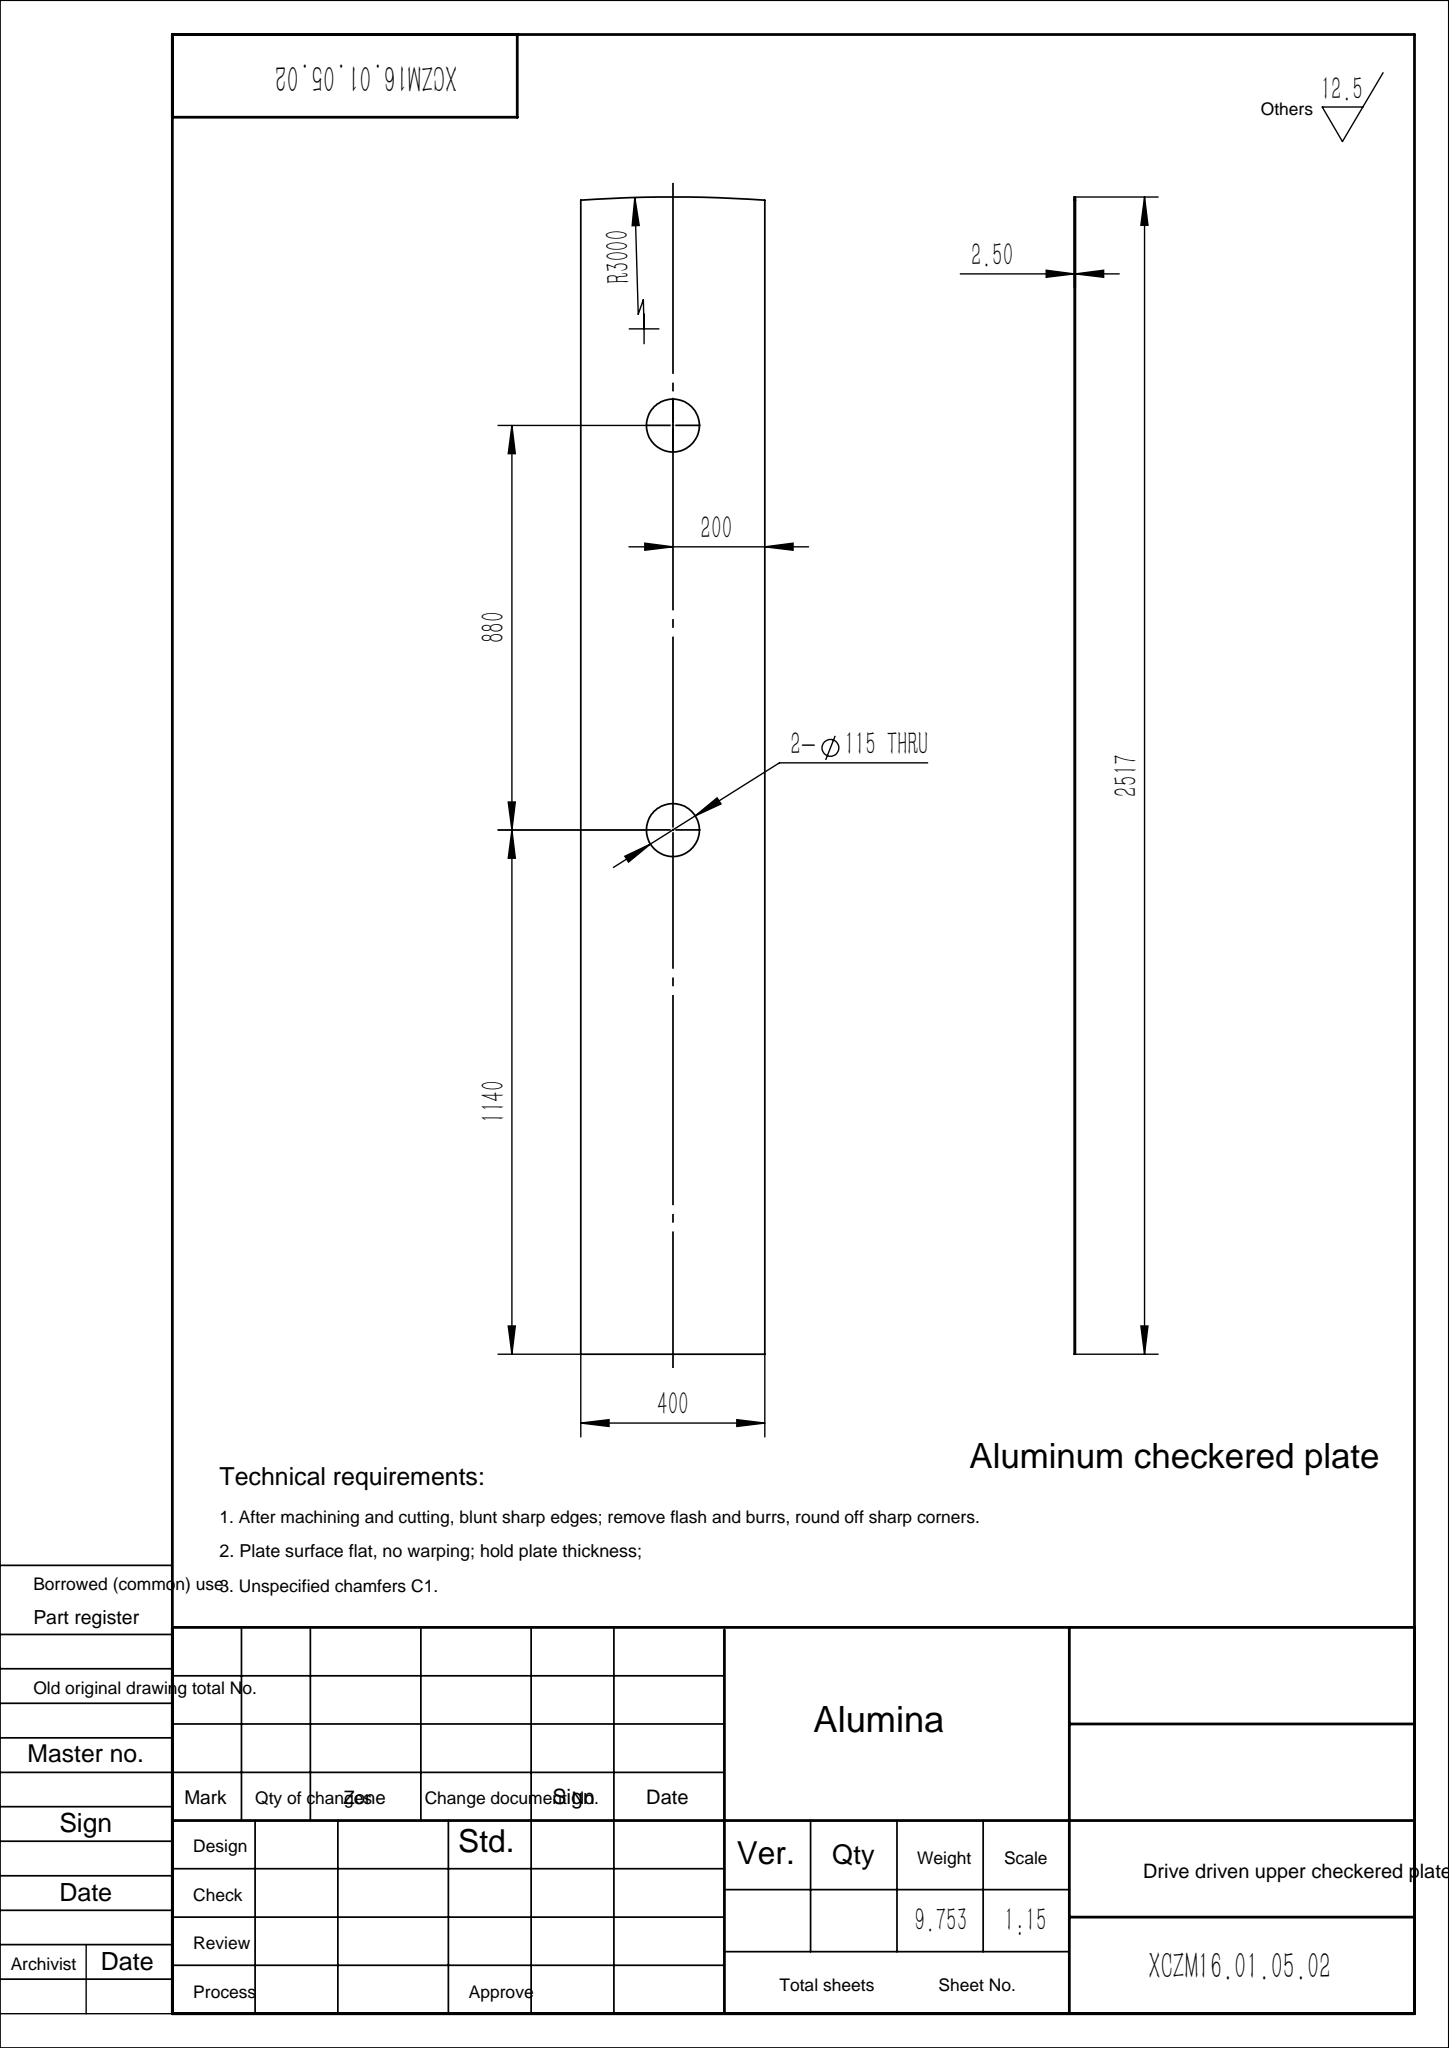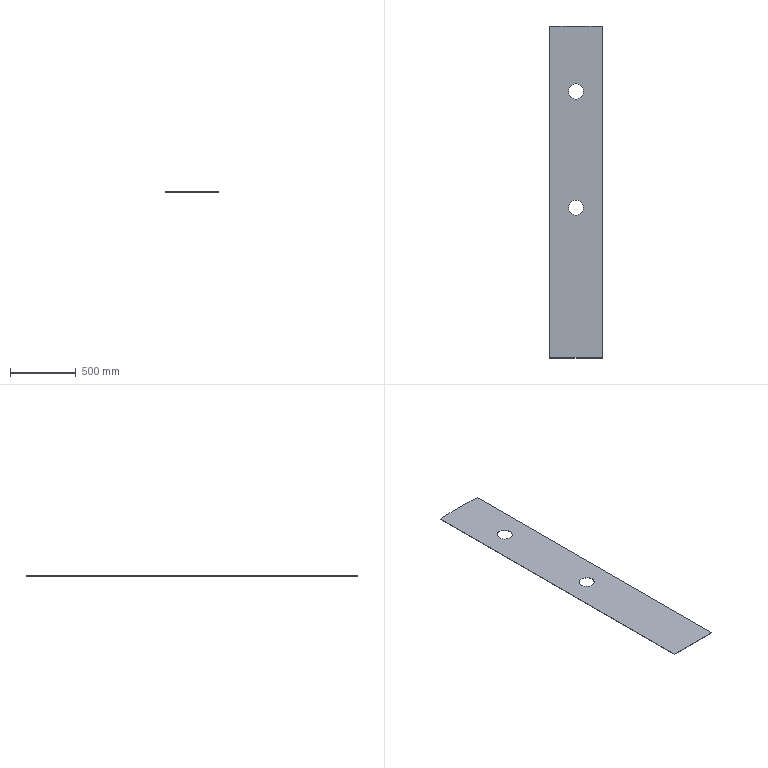Part | SolidWorks | features Extrusion 1 | 1 solid | 10 faces | box 400 x 2517 x 2.5 mm | volume 2462842 mm3 | cylinder 5 | plane 5 | commonest cylinder face diameters 115 x4 6000 x1
STEP:
#1=CARTESIAN_POINT('',(-57.5,1140.,2.5));
#2=VERTEX_POINT('',#1);
#3=CARTESIAN_POINT('',(57.5,1140.,2.5));
#4=VERTEX_POINT('',#3);
#5=CARTESIAN_POINT('',(0.,1140.,2.5));
#6=DIRECTION('',(0.,0.,1.));
#7=DIRECTION('',(1.,0.,0.));
#8=AXIS2_PLACEMENT_3D('',#5,#6,#7);
#9=CIRCLE('',#8,57.5);
#10=EDGE_CURVE('',#2,#4,#9,.T.);
#11=ORIENTED_EDGE('',*,*,#10,.T.);
#12=CARTESIAN_POINT('',(57.5,1140.,0.));
#13=VERTEX_POINT('',#12);
#14=CARTESIAN_POINT('',(57.5,1140.,2.5));
#15=DIRECTION('',(0.,0.,-1.));
#16=VECTOR('',#15,1000.);
#17=LINE('',#14,#16);
#18=EDGE_CURVE('',#4,#13,#17,.T.);
#19=ORIENTED_EDGE('',*,*,#18,.T.);
#20=CARTESIAN_POINT('',(-57.5,1140.,0.));
#21=VERTEX_POINT('',#20);
#22=CARTESIAN_POINT('',(0.,1140.,0.));
#23=DIRECTION('',(0.,0.,1.));
#24=DIRECTION('',(1.,0.,0.));
#25=AXIS2_PLACEMENT_3D('',#22,#23,#24);
#26=CIRCLE('',#25,57.5);
#27=EDGE_CURVE('',#21,#13,#26,.T.);
#28=ORIENTED_EDGE('',*,*,#27,.F.);
#29=CARTESIAN_POINT('',(-57.5,1140.,2.5));
#30=DIRECTION('',(0.,0.,-1.));
#31=VECTOR('',#30,1000.);
#32=LINE('',#29,#31);
#33=EDGE_CURVE('',#2,#21,#32,.T.);
#34=ORIENTED_EDGE('',*,*,#33,.F.);
#35=EDGE_LOOP('',(#11,#19,#28,#34));
#36=FACE_OUTER_BOUND('',#35,.T.);
#37=CARTESIAN_POINT('',(0.,1140.,2.5));
#38=DIRECTION('',(0.,0.,-1.));
#39=DIRECTION('',(-1.,0.,0.));
#40=AXIS2_PLACEMENT_3D('',#37,#38,#39);
#41=CYLINDRICAL_SURFACE('',#40,57.5);
#42=ADVANCED_FACE('',(#36),#41,.F.);
#43=CARTESIAN_POINT('',(-57.5,2020.,2.5));
#44=VERTEX_POINT('',#43);
#45=CARTESIAN_POINT('',(57.5,2020.,2.5));
#46=VERTEX_POINT('',#45);
#47=CARTESIAN_POINT('',(0.,2020.,2.5));
#48=DIRECTION('',(0.,0.,1.));
#49=DIRECTION('',(1.,0.,0.));
#50=AXIS2_PLACEMENT_3D('',#47,#48,#49);
#51=CIRCLE('',#50,57.5);
#52=EDGE_CURVE('',#44,#46,#51,.T.);
#53=ORIENTED_EDGE('',*,*,#52,.T.);
#54=CARTESIAN_POINT('',(57.5,2020.,0.));
#55=VERTEX_POINT('',#54);
#56=CARTESIAN_POINT('',(57.5,2020.,2.5));
#57=DIRECTION('',(0.,0.,-1.));
#58=VECTOR('',#57,1000.);
#59=LINE('',#56,#58);
#60=EDGE_CURVE('',#46,#55,#59,.T.);
#61=ORIENTED_EDGE('',*,*,#60,.T.);
#62=CARTESIAN_POINT('',(-57.5,2020.,0.));
#63=VERTEX_POINT('',#62);
#64=CARTESIAN_POINT('',(0.,2020.,0.));
#65=DIRECTION('',(0.,0.,1.));
#66=DIRECTION('',(1.,0.,0.));
#67=AXIS2_PLACEMENT_3D('',#64,#65,#66);
#68=CIRCLE('',#67,57.5);
#69=EDGE_CURVE('',#63,#55,#68,.T.);
#70=ORIENTED_EDGE('',*,*,#69,.F.);
#71=CARTESIAN_POINT('',(-57.5,2020.,2.5));
#72=DIRECTION('',(0.,0.,-1.));
#73=VECTOR('',#72,1000.);
#74=LINE('',#71,#73);
#75=EDGE_CURVE('',#44,#63,#74,.T.);
#76=ORIENTED_EDGE('',*,*,#75,.F.);
#77=EDGE_LOOP('',(#53,#61,#70,#76));
#78=FACE_OUTER_BOUND('',#77,.T.);
#79=CARTESIAN_POINT('',(0.,2020.,2.5));
#80=DIRECTION('',(0.,0.,-1.));
#81=DIRECTION('',(-1.,0.,0.));
#82=AXIS2_PLACEMENT_3D('',#79,#80,#81);
#83=CYLINDRICAL_SURFACE('',#82,57.5);
#84=ADVANCED_FACE('',(#78),#83,.F.);
#85=ORIENTED_EDGE('',*,*,#52,.F.);
#86=CARTESIAN_POINT('',(0.,2020.,2.5));
#87=DIRECTION('',(0.,0.,1.));
#88=DIRECTION('',(1.,0.,0.));
#89=AXIS2_PLACEMENT_3D('',#86,#87,#88);
#90=CIRCLE('',#89,57.5);
#91=EDGE_CURVE('',#46,#44,#90,.T.);
#92=ORIENTED_EDGE('',*,*,#91,.F.);
#93=EDGE_LOOP('',(#85,#92));
#94=FACE_BOUND('',#93,.T.);
#95=CARTESIAN_POINT('',(200.,0.,2.5));
#96=VERTEX_POINT('',#95);
#97=CARTESIAN_POINT('',(200.,2510.326,2.5));
#98=VERTEX_POINT('',#97);
#99=CARTESIAN_POINT('',(200.,0.,2.5));
#100=DIRECTION('',(0.,1.,0.));
#101=VECTOR('',#100,1000.);
#102=LINE('',#99,#101);
#103=EDGE_CURVE('',#96,#98,#102,.T.);
#104=ORIENTED_EDGE('',*,*,#103,.T.);
#105=CARTESIAN_POINT('',(-200.,2510.326,2.5));
#106=VERTEX_POINT('',#105);
#107=CARTESIAN_POINT('',(0.,-483.,2.5));
#108=DIRECTION('',(0.,0.,1.));
#109=DIRECTION('',(1.,0.,0.));
#110=AXIS2_PLACEMENT_3D('',#107,#108,#109);
#111=CIRCLE('',#110,3000.);
#112=EDGE_CURVE('',#98,#106,#111,.T.);
#113=ORIENTED_EDGE('',*,*,#112,.T.);
#114=CARTESIAN_POINT('',(-200.,0.,2.5));
#115=VERTEX_POINT('',#114);
#116=CARTESIAN_POINT('',(-200.,0.,2.5));
#117=DIRECTION('',(0.,-1.,0.));
#118=VECTOR('',#117,1000.);
#119=LINE('',#116,#118);
#120=EDGE_CURVE('',#106,#115,#119,.T.);
#121=ORIENTED_EDGE('',*,*,#120,.T.);
#122=CARTESIAN_POINT('',(-200.,0.,2.5));
#123=DIRECTION('',(1.,0.,0.));
#124=VECTOR('',#123,1000.);
#125=LINE('',#122,#124);
#126=EDGE_CURVE('',#115,#96,#125,.T.);
#127=ORIENTED_EDGE('',*,*,#126,.T.);
#128=EDGE_LOOP('',(#104,#113,#121,#127));
#129=FACE_OUTER_BOUND('',#128,.T.);
#130=ORIENTED_EDGE('',*,*,#10,.F.);
#131=CARTESIAN_POINT('',(0.,1140.,2.5));
#132=DIRECTION('',(0.,0.,1.));
#133=DIRECTION('',(1.,0.,0.));
#134=AXIS2_PLACEMENT_3D('',#131,#132,#133);
#135=CIRCLE('',#134,57.5);
#136=EDGE_CURVE('',#4,#2,#135,.T.);
#137=ORIENTED_EDGE('',*,*,#136,.F.);
#138=EDGE_LOOP('',(#130,#137));
#139=FACE_BOUND('',#138,.T.);
#140=CARTESIAN_POINT('',(0.,-483.,2.5));
#141=DIRECTION('',(0.,0.,1.));
#142=DIRECTION('',(1.,0.,0.));
#143=AXIS2_PLACEMENT_3D('',#140,#141,#142);
#144=PLANE('',#143);
#145=ADVANCED_FACE('',(#94,#129,#139),#144,.T.);
#146=CARTESIAN_POINT('',(200.,0.,0.));
#147=VERTEX_POINT('',#146);
#148=CARTESIAN_POINT('',(200.,2510.326,0.));
#149=VERTEX_POINT('',#148);
#150=CARTESIAN_POINT('',(200.,0.,0.));
#151=DIRECTION('',(0.,1.,0.));
#152=VECTOR('',#151,1000.);
#153=LINE('',#150,#152);
#154=EDGE_CURVE('',#147,#149,#153,.T.);
#155=ORIENTED_EDGE('',*,*,#154,.F.);
#156=CARTESIAN_POINT('',(-200.,0.,0.));
#157=VERTEX_POINT('',#156);
#158=CARTESIAN_POINT('',(-200.,0.,0.));
#159=DIRECTION('',(1.,0.,0.));
#160=VECTOR('',#159,1000.);
#161=LINE('',#158,#160);
#162=EDGE_CURVE('',#157,#147,#161,.T.);
#163=ORIENTED_EDGE('',*,*,#162,.F.);
#164=CARTESIAN_POINT('',(-200.,2510.326,0.));
#165=VERTEX_POINT('',#164);
#166=CARTESIAN_POINT('',(-200.,0.,0.));
#167=DIRECTION('',(0.,-1.,0.));
#168=VECTOR('',#167,1000.);
#169=LINE('',#166,#168);
#170=EDGE_CURVE('',#165,#157,#169,.T.);
#171=ORIENTED_EDGE('',*,*,#170,.F.);
#172=CARTESIAN_POINT('',(0.,-483.,0.));
#173=DIRECTION('',(0.,0.,1.));
#174=DIRECTION('',(1.,0.,0.));
#175=AXIS2_PLACEMENT_3D('',#172,#173,#174);
#176=CIRCLE('',#175,3000.);
#177=EDGE_CURVE('',#149,#165,#176,.T.);
#178=ORIENTED_EDGE('',*,*,#177,.F.);
#179=EDGE_LOOP('',(#155,#163,#171,#178));
#180=FACE_OUTER_BOUND('',#179,.T.);
#181=ORIENTED_EDGE('',*,*,#69,.T.);
#182=CARTESIAN_POINT('',(0.,2020.,0.));
#183=DIRECTION('',(0.,0.,1.));
#184=DIRECTION('',(1.,0.,0.));
#185=AXIS2_PLACEMENT_3D('',#182,#183,#184);
#186=CIRCLE('',#185,57.5);
#187=EDGE_CURVE('',#55,#63,#186,.T.);
#188=ORIENTED_EDGE('',*,*,#187,.T.);
#189=EDGE_LOOP('',(#181,#188));
#190=FACE_BOUND('',#189,.T.);
#191=ORIENTED_EDGE('',*,*,#27,.T.);
#192=CARTESIAN_POINT('',(0.,1140.,0.));
#193=DIRECTION('',(0.,0.,1.));
#194=DIRECTION('',(1.,0.,0.));
#195=AXIS2_PLACEMENT_3D('',#192,#193,#194);
#196=CIRCLE('',#195,57.5);
#197=EDGE_CURVE('',#13,#21,#196,.T.);
#198=ORIENTED_EDGE('',*,*,#197,.T.);
#199=EDGE_LOOP('',(#191,#198));
#200=FACE_BOUND('',#199,.T.);
#201=CARTESIAN_POINT('',(0.,-483.,0.));
#202=DIRECTION('',(0.,0.,1.));
#203=DIRECTION('',(1.,0.,0.));
#204=AXIS2_PLACEMENT_3D('',#201,#202,#203);
#205=PLANE('',#204);
#206=ADVANCED_FACE('',(#180,#190,#200),#205,.F.);
#207=ORIENTED_EDGE('',*,*,#154,.T.);
#208=CARTESIAN_POINT('',(200.,2510.326,2.5));
#209=DIRECTION('',(0.,0.,-1.));
#210=VECTOR('',#209,1000.);
#211=LINE('',#208,#210);
#212=EDGE_CURVE('',#98,#149,#211,.T.);
#213=ORIENTED_EDGE('',*,*,#212,.F.);
#214=ORIENTED_EDGE('',*,*,#103,.F.);
#215=CARTESIAN_POINT('',(200.,0.,2.5));
#216=DIRECTION('',(0.,0.,-1.));
#217=VECTOR('',#216,1000.);
#218=LINE('',#215,#217);
#219=EDGE_CURVE('',#96,#147,#218,.T.);
#220=ORIENTED_EDGE('',*,*,#219,.T.);
#221=EDGE_LOOP('',(#207,#213,#214,#220));
#222=FACE_OUTER_BOUND('',#221,.T.);
#223=CARTESIAN_POINT('',(200.,0.,2.5));
#224=DIRECTION('',(-1.,0.,0.));
#225=DIRECTION('',(0.,-1.,0.));
#226=AXIS2_PLACEMENT_3D('',#223,#224,#225);
#227=PLANE('',#226);
#228=ADVANCED_FACE('',(#222),#227,.F.);
#229=ORIENTED_EDGE('',*,*,#177,.T.);
#230=CARTESIAN_POINT('',(-200.,2510.326,2.5));
#231=DIRECTION('',(0.,0.,-1.));
#232=VECTOR('',#231,1000.);
#233=LINE('',#230,#232);
#234=EDGE_CURVE('',#106,#165,#233,.T.);
#235=ORIENTED_EDGE('',*,*,#234,.F.);
#236=ORIENTED_EDGE('',*,*,#112,.F.);
#237=ORIENTED_EDGE('',*,*,#212,.T.);
#238=EDGE_LOOP('',(#229,#235,#236,#237));
#239=FACE_OUTER_BOUND('',#238,.T.);
#240=CARTESIAN_POINT('',(0.,-483.,2.5));
#241=DIRECTION('',(0.,0.,-1.));
#242=DIRECTION('',(-1.,0.,0.));
#243=AXIS2_PLACEMENT_3D('',#240,#241,#242);
#244=CYLINDRICAL_SURFACE('',#243,3000.);
#245=ADVANCED_FACE('',(#239),#244,.T.);
#246=ORIENTED_EDGE('',*,*,#170,.T.);
#247=CARTESIAN_POINT('',(-200.,0.,2.5));
#248=DIRECTION('',(0.,0.,-1.));
#249=VECTOR('',#248,1000.);
#250=LINE('',#247,#249);
#251=EDGE_CURVE('',#115,#157,#250,.T.);
#252=ORIENTED_EDGE('',*,*,#251,.F.);
#253=ORIENTED_EDGE('',*,*,#120,.F.);
#254=ORIENTED_EDGE('',*,*,#234,.T.);
#255=EDGE_LOOP('',(#246,#252,#253,#254));
#256=FACE_OUTER_BOUND('',#255,.T.);
#257=CARTESIAN_POINT('',(-200.,0.,2.5));
#258=DIRECTION('',(1.,0.,0.));
#259=DIRECTION('',(0.,1.,0.));
#260=AXIS2_PLACEMENT_3D('',#257,#258,#259);
#261=PLANE('',#260);
#262=ADVANCED_FACE('',(#256),#261,.F.);
#263=ORIENTED_EDGE('',*,*,#162,.T.);
#264=ORIENTED_EDGE('',*,*,#219,.F.);
#265=ORIENTED_EDGE('',*,*,#126,.F.);
#266=ORIENTED_EDGE('',*,*,#251,.T.);
#267=EDGE_LOOP('',(#263,#264,#265,#266));
#268=FACE_OUTER_BOUND('',#267,.T.);
#269=CARTESIAN_POINT('',(-200.,0.,2.5));
#270=DIRECTION('',(0.,1.,0.));
#271=DIRECTION('',(0.,0.,1.));
#272=AXIS2_PLACEMENT_3D('',#269,#270,#271);
#273=PLANE('',#272);
#274=ADVANCED_FACE('',(#268),#273,.F.);
#275=ORIENTED_EDGE('',*,*,#60,.F.);
#276=ORIENTED_EDGE('',*,*,#91,.T.);
#277=ORIENTED_EDGE('',*,*,#75,.T.);
#278=ORIENTED_EDGE('',*,*,#187,.F.);
#279=EDGE_LOOP('',(#275,#276,#277,#278));
#280=FACE_OUTER_BOUND('',#279,.T.);
#281=CARTESIAN_POINT('',(0.,2020.,2.5));
#282=DIRECTION('',(0.,0.,-1.));
#283=DIRECTION('',(-1.,0.,0.));
#284=AXIS2_PLACEMENT_3D('',#281,#282,#283);
#285=CYLINDRICAL_SURFACE('',#284,57.5);
#286=ADVANCED_FACE('',(#280),#285,.F.);
#287=ORIENTED_EDGE('',*,*,#18,.F.);
#288=ORIENTED_EDGE('',*,*,#136,.T.);
#289=ORIENTED_EDGE('',*,*,#33,.T.);
#290=ORIENTED_EDGE('',*,*,#197,.F.);
#291=EDGE_LOOP('',(#287,#288,#289,#290));
#292=FACE_OUTER_BOUND('',#291,.T.);
#293=CARTESIAN_POINT('',(0.,1140.,2.5));
#294=DIRECTION('',(0.,0.,-1.));
#295=DIRECTION('',(-1.,0.,0.));
#296=AXIS2_PLACEMENT_3D('',#293,#294,#295);
#297=CYLINDRICAL_SURFACE('',#296,57.5);
#298=ADVANCED_FACE('',(#292),#297,.F.);
#299=CLOSED_SHELL('',(#42,#84,#145,#206,#228,#245,#262,#274,#286,#298));
#300=MANIFOLD_SOLID_BREP('',#299);
#301=CARTESIAN_POINT('',(0.,0.,0.));
#302=DIRECTION('',(0.,0.,1.));
#303=DIRECTION('',(1.,0.,0.));
#304=AXIS2_PLACEMENT_3D('',#301,#302,#303);
#305=(LENGTH_UNIT()NAMED_UNIT(*)SI_UNIT(.MILLI.,.METRE.));
#306=UNCERTAINTY_MEASURE_WITH_UNIT(LENGTH_MEASURE(0.00001),#305,'','');
#307=(NAMED_UNIT(*)PLANE_ANGLE_UNIT()SI_UNIT($,.RADIAN.));
#308=(NAMED_UNIT(*)SI_UNIT($,.STERADIAN.)SOLID_ANGLE_UNIT());
#309=(GEOMETRIC_REPRESENTATION_CONTEXT(3)GLOBAL_UNCERTAINTY_ASSIGNED_CONTEXT((#306))GLOBAL_UNIT_ASSIGNED_CONTEXT((#305,#307,#308))REPRESENTATION_CONTEXT('',''));
#310=ADVANCED_BREP_SHAPE_REPRESENTATION('',(#300,#304),#309);